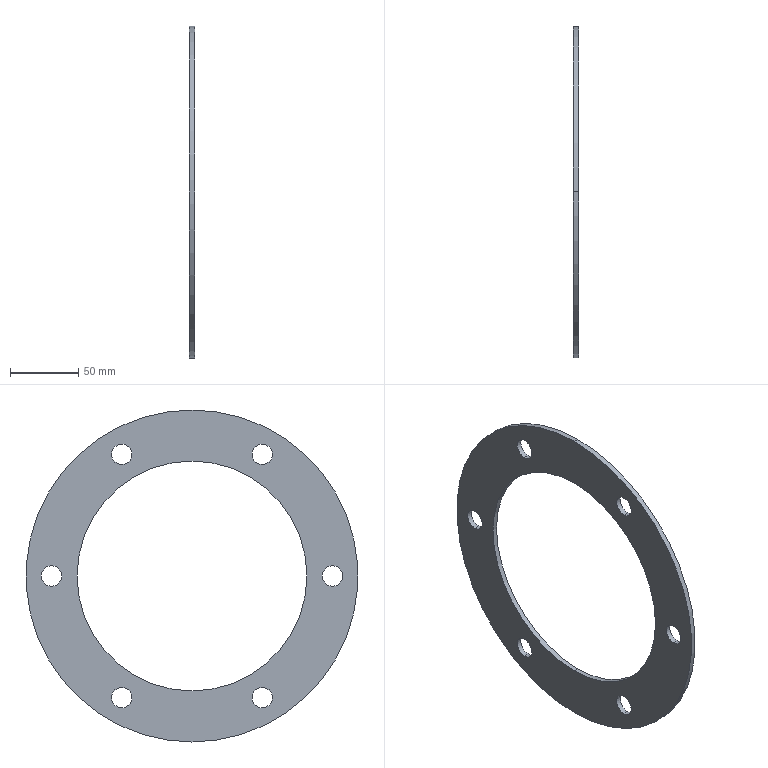Part | SolidWorks | features ICE 1, Revolution 1, Scale 1 | 1 solid | 18 faces | box 3.75 x 243.75 x 243.75 mm | volume 87142 mm3 | cylinder 16 | plane 2 | commonest cylinder face diameters 15 x12 168.75 x2 243.75 x2
STEP:
#1=CARTESIAN_POINT('',(-0.875,-103.125,7.5));
#2=VERTEX_POINT('',#1);
#3=CARTESIAN_POINT('',(-0.875,-103.125,-7.5));
#4=VERTEX_POINT('',#3);
#5=CARTESIAN_POINT('',(-0.875,-103.125,0.));
#6=DIRECTION('',(1.,0.,0.));
#7=DIRECTION('',(0.,0.,-1.));
#8=AXIS2_PLACEMENT_3D('',#5,#6,#7);
#9=CIRCLE('',#8,7.5);
#10=EDGE_CURVE('',#2,#4,#9,.T.);
#11=ORIENTED_EDGE('',*,*,#10,.F.);
#12=CARTESIAN_POINT('',(2.875,-103.125,7.5));
#13=VERTEX_POINT('',#12);
#14=CARTESIAN_POINT('',(-15.875,-103.125,7.5));
#15=DIRECTION('',(1.,0.,0.));
#16=VECTOR('',#15,1000.);
#17=LINE('',#14,#16);
#18=EDGE_CURVE('',#2,#13,#17,.T.);
#19=ORIENTED_EDGE('',*,*,#18,.T.);
#20=CARTESIAN_POINT('',(2.875,-103.125,-7.5));
#21=VERTEX_POINT('',#20);
#22=CARTESIAN_POINT('',(2.875,-103.125,0.));
#23=DIRECTION('',(1.,0.,0.));
#24=DIRECTION('',(0.,0.,1.));
#25=AXIS2_PLACEMENT_3D('',#22,#23,#24);
#26=CIRCLE('',#25,7.5);
#27=EDGE_CURVE('',#13,#21,#26,.T.);
#28=ORIENTED_EDGE('',*,*,#27,.T.);
#29=CARTESIAN_POINT('',(-15.875,-103.125,-7.5));
#30=DIRECTION('',(1.,0.,0.));
#31=VECTOR('',#30,1000.);
#32=LINE('',#29,#31);
#33=EDGE_CURVE('',#4,#21,#32,.T.);
#34=ORIENTED_EDGE('',*,*,#33,.F.);
#35=EDGE_LOOP('',(#11,#19,#28,#34));
#36=FACE_OUTER_BOUND('',#35,.T.);
#37=CARTESIAN_POINT('',(-15.875,-103.125,0.));
#38=DIRECTION('',(1.,0.,0.));
#39=DIRECTION('',(0.,0.,-1.));
#40=AXIS2_PLACEMENT_3D('',#37,#38,#39);
#41=CYLINDRICAL_SURFACE('',#40,7.5);
#42=ADVANCED_FACE('',(#36),#41,.F.);
#43=CARTESIAN_POINT('',(-0.875,-51.562,96.809));
#44=VERTEX_POINT('',#43);
#45=CARTESIAN_POINT('',(-0.875,-51.562,81.809));
#46=VERTEX_POINT('',#45);
#47=CARTESIAN_POINT('',(-0.875,-51.562,89.309));
#48=DIRECTION('',(1.,0.,0.));
#49=DIRECTION('',(0.,0.,-1.));
#50=AXIS2_PLACEMENT_3D('',#47,#48,#49);
#51=CIRCLE('',#50,7.5);
#52=EDGE_CURVE('',#44,#46,#51,.T.);
#53=ORIENTED_EDGE('',*,*,#52,.F.);
#54=CARTESIAN_POINT('',(2.875,-51.562,96.809));
#55=VERTEX_POINT('',#54);
#56=CARTESIAN_POINT('',(-15.875,-51.562,96.809));
#57=DIRECTION('',(1.,0.,0.));
#58=VECTOR('',#57,1000.);
#59=LINE('',#56,#58);
#60=EDGE_CURVE('',#44,#55,#59,.T.);
#61=ORIENTED_EDGE('',*,*,#60,.T.);
#62=CARTESIAN_POINT('',(2.875,-51.562,81.809));
#63=VERTEX_POINT('',#62);
#64=CARTESIAN_POINT('',(2.875,-51.562,89.309));
#65=DIRECTION('',(1.,0.,0.));
#66=DIRECTION('',(0.,0.,1.));
#67=AXIS2_PLACEMENT_3D('',#64,#65,#66);
#68=CIRCLE('',#67,7.5);
#69=EDGE_CURVE('',#55,#63,#68,.T.);
#70=ORIENTED_EDGE('',*,*,#69,.T.);
#71=CARTESIAN_POINT('',(-15.875,-51.562,81.809));
#72=DIRECTION('',(1.,0.,0.));
#73=VECTOR('',#72,1000.);
#74=LINE('',#71,#73);
#75=EDGE_CURVE('',#46,#63,#74,.T.);
#76=ORIENTED_EDGE('',*,*,#75,.F.);
#77=EDGE_LOOP('',(#53,#61,#70,#76));
#78=FACE_OUTER_BOUND('',#77,.T.);
#79=CARTESIAN_POINT('',(-15.875,-51.562,89.309));
#80=DIRECTION('',(1.,0.,0.));
#81=DIRECTION('',(0.,0.,-1.));
#82=AXIS2_PLACEMENT_3D('',#79,#80,#81);
#83=CYLINDRICAL_SURFACE('',#82,7.5);
#84=ADVANCED_FACE('',(#78),#83,.F.);
#85=CARTESIAN_POINT('',(-0.875,-51.562,-81.809));
#86=VERTEX_POINT('',#85);
#87=CARTESIAN_POINT('',(-0.875,-51.562,-96.809));
#88=VERTEX_POINT('',#87);
#89=CARTESIAN_POINT('',(-0.875,-51.562,-89.309));
#90=DIRECTION('',(1.,0.,0.));
#91=DIRECTION('',(0.,0.,-1.));
#92=AXIS2_PLACEMENT_3D('',#89,#90,#91);
#93=CIRCLE('',#92,7.5);
#94=EDGE_CURVE('',#86,#88,#93,.T.);
#95=ORIENTED_EDGE('',*,*,#94,.F.);
#96=CARTESIAN_POINT('',(2.875,-51.562,-81.809));
#97=VERTEX_POINT('',#96);
#98=CARTESIAN_POINT('',(-15.875,-51.562,-81.809));
#99=DIRECTION('',(1.,0.,0.));
#100=VECTOR('',#99,1000.);
#101=LINE('',#98,#100);
#102=EDGE_CURVE('',#86,#97,#101,.T.);
#103=ORIENTED_EDGE('',*,*,#102,.T.);
#104=CARTESIAN_POINT('',(2.875,-51.562,-96.809));
#105=VERTEX_POINT('',#104);
#106=CARTESIAN_POINT('',(2.875,-51.562,-89.309));
#107=DIRECTION('',(1.,0.,0.));
#108=DIRECTION('',(0.,0.,1.));
#109=AXIS2_PLACEMENT_3D('',#106,#107,#108);
#110=CIRCLE('',#109,7.5);
#111=EDGE_CURVE('',#97,#105,#110,.T.);
#112=ORIENTED_EDGE('',*,*,#111,.T.);
#113=CARTESIAN_POINT('',(-15.875,-51.562,-96.809));
#114=DIRECTION('',(1.,0.,0.));
#115=VECTOR('',#114,1000.);
#116=LINE('',#113,#115);
#117=EDGE_CURVE('',#88,#105,#116,.T.);
#118=ORIENTED_EDGE('',*,*,#117,.F.);
#119=EDGE_LOOP('',(#95,#103,#112,#118));
#120=FACE_OUTER_BOUND('',#119,.T.);
#121=CARTESIAN_POINT('',(-15.875,-51.562,-89.309));
#122=DIRECTION('',(1.,0.,0.));
#123=DIRECTION('',(0.,0.,-1.));
#124=AXIS2_PLACEMENT_3D('',#121,#122,#123);
#125=CYLINDRICAL_SURFACE('',#124,7.5);
#126=ADVANCED_FACE('',(#120),#125,.F.);
#127=CARTESIAN_POINT('',(-0.875,51.562,96.809));
#128=VERTEX_POINT('',#127);
#129=CARTESIAN_POINT('',(-0.875,51.562,81.809));
#130=VERTEX_POINT('',#129);
#131=CARTESIAN_POINT('',(-0.875,51.562,89.309));
#132=DIRECTION('',(1.,0.,0.));
#133=DIRECTION('',(0.,0.,-1.));
#134=AXIS2_PLACEMENT_3D('',#131,#132,#133);
#135=CIRCLE('',#134,7.5);
#136=EDGE_CURVE('',#128,#130,#135,.T.);
#137=ORIENTED_EDGE('',*,*,#136,.F.);
#138=CARTESIAN_POINT('',(2.875,51.562,96.809));
#139=VERTEX_POINT('',#138);
#140=CARTESIAN_POINT('',(-15.875,51.562,96.809));
#141=DIRECTION('',(1.,0.,0.));
#142=VECTOR('',#141,1000.);
#143=LINE('',#140,#142);
#144=EDGE_CURVE('',#128,#139,#143,.T.);
#145=ORIENTED_EDGE('',*,*,#144,.T.);
#146=CARTESIAN_POINT('',(2.875,51.562,81.809));
#147=VERTEX_POINT('',#146);
#148=CARTESIAN_POINT('',(2.875,51.562,89.309));
#149=DIRECTION('',(1.,0.,0.));
#150=DIRECTION('',(0.,0.,-1.));
#151=AXIS2_PLACEMENT_3D('',#148,#149,#150);
#152=CIRCLE('',#151,7.5);
#153=EDGE_CURVE('',#139,#147,#152,.T.);
#154=ORIENTED_EDGE('',*,*,#153,.T.);
#155=CARTESIAN_POINT('',(-15.875,51.562,81.809));
#156=DIRECTION('',(1.,0.,0.));
#157=VECTOR('',#156,1000.);
#158=LINE('',#155,#157);
#159=EDGE_CURVE('',#130,#147,#158,.T.);
#160=ORIENTED_EDGE('',*,*,#159,.F.);
#161=EDGE_LOOP('',(#137,#145,#154,#160));
#162=FACE_OUTER_BOUND('',#161,.T.);
#163=CARTESIAN_POINT('',(-15.875,51.562,89.309));
#164=DIRECTION('',(1.,0.,0.));
#165=DIRECTION('',(0.,0.,-1.));
#166=AXIS2_PLACEMENT_3D('',#163,#164,#165);
#167=CYLINDRICAL_SURFACE('',#166,7.5);
#168=ADVANCED_FACE('',(#162),#167,.F.);
#169=CARTESIAN_POINT('',(-0.875,51.562,-81.809));
#170=VERTEX_POINT('',#169);
#171=CARTESIAN_POINT('',(-0.875,51.562,-96.809));
#172=VERTEX_POINT('',#171);
#173=CARTESIAN_POINT('',(-0.875,51.562,-89.309));
#174=DIRECTION('',(1.,0.,0.));
#175=DIRECTION('',(0.,0.,-1.));
#176=AXIS2_PLACEMENT_3D('',#173,#174,#175);
#177=CIRCLE('',#176,7.5);
#178=EDGE_CURVE('',#170,#172,#177,.T.);
#179=ORIENTED_EDGE('',*,*,#178,.F.);
#180=CARTESIAN_POINT('',(2.875,51.562,-81.809));
#181=VERTEX_POINT('',#180);
#182=CARTESIAN_POINT('',(-15.875,51.562,-81.809));
#183=DIRECTION('',(1.,0.,0.));
#184=VECTOR('',#183,1000.);
#185=LINE('',#182,#184);
#186=EDGE_CURVE('',#170,#181,#185,.T.);
#187=ORIENTED_EDGE('',*,*,#186,.T.);
#188=CARTESIAN_POINT('',(2.875,51.562,-96.809));
#189=VERTEX_POINT('',#188);
#190=CARTESIAN_POINT('',(2.875,51.562,-89.309));
#191=DIRECTION('',(1.,0.,0.));
#192=DIRECTION('',(0.,0.,-1.));
#193=AXIS2_PLACEMENT_3D('',#190,#191,#192);
#194=CIRCLE('',#193,7.5);
#195=EDGE_CURVE('',#181,#189,#194,.T.);
#196=ORIENTED_EDGE('',*,*,#195,.T.);
#197=CARTESIAN_POINT('',(-15.875,51.562,-96.809));
#198=DIRECTION('',(1.,0.,0.));
#199=VECTOR('',#198,1000.);
#200=LINE('',#197,#199);
#201=EDGE_CURVE('',#172,#189,#200,.T.);
#202=ORIENTED_EDGE('',*,*,#201,.F.);
#203=EDGE_LOOP('',(#179,#187,#196,#202));
#204=FACE_OUTER_BOUND('',#203,.T.);
#205=CARTESIAN_POINT('',(-15.875,51.562,-89.309));
#206=DIRECTION('',(1.,0.,0.));
#207=DIRECTION('',(0.,0.,-1.));
#208=AXIS2_PLACEMENT_3D('',#205,#206,#207);
#209=CYLINDRICAL_SURFACE('',#208,7.5);
#210=ADVANCED_FACE('',(#204),#209,.F.);
#211=CARTESIAN_POINT('',(-0.875,103.125,7.5));
#212=VERTEX_POINT('',#211);
#213=CARTESIAN_POINT('',(-0.875,103.125,-7.5));
#214=VERTEX_POINT('',#213);
#215=CARTESIAN_POINT('',(-0.875,103.125,0.));
#216=DIRECTION('',(1.,0.,0.));
#217=DIRECTION('',(0.,0.,-1.));
#218=AXIS2_PLACEMENT_3D('',#215,#216,#217);
#219=CIRCLE('',#218,7.5);
#220=EDGE_CURVE('',#212,#214,#219,.T.);
#221=ORIENTED_EDGE('',*,*,#220,.F.);
#222=CARTESIAN_POINT('',(2.875,103.125,7.5));
#223=VERTEX_POINT('',#222);
#224=CARTESIAN_POINT('',(-15.875,103.125,7.5));
#225=DIRECTION('',(1.,0.,0.));
#226=VECTOR('',#225,1000.);
#227=LINE('',#224,#226);
#228=EDGE_CURVE('',#212,#223,#227,.T.);
#229=ORIENTED_EDGE('',*,*,#228,.T.);
#230=CARTESIAN_POINT('',(2.875,103.125,-7.5));
#231=VERTEX_POINT('',#230);
#232=CARTESIAN_POINT('',(2.875,103.125,0.));
#233=DIRECTION('',(1.,0.,0.));
#234=DIRECTION('',(0.,0.,-1.));
#235=AXIS2_PLACEMENT_3D('',#232,#233,#234);
#236=CIRCLE('',#235,7.5);
#237=EDGE_CURVE('',#223,#231,#236,.T.);
#238=ORIENTED_EDGE('',*,*,#237,.T.);
#239=CARTESIAN_POINT('',(-15.875,103.125,-7.5));
#240=DIRECTION('',(1.,0.,0.));
#241=VECTOR('',#240,1000.);
#242=LINE('',#239,#241);
#243=EDGE_CURVE('',#214,#231,#242,.T.);
#244=ORIENTED_EDGE('',*,*,#243,.F.);
#245=EDGE_LOOP('',(#221,#229,#238,#244));
#246=FACE_OUTER_BOUND('',#245,.T.);
#247=CARTESIAN_POINT('',(-15.875,103.125,0.));
#248=DIRECTION('',(1.,0.,0.));
#249=DIRECTION('',(0.,0.,-1.));
#250=AXIS2_PLACEMENT_3D('',#247,#248,#249);
#251=CYLINDRICAL_SURFACE('',#250,7.5);
#252=ADVANCED_FACE('',(#246),#251,.F.);
#253=CARTESIAN_POINT('',(2.875,0.,121.875));
#254=VERTEX_POINT('',#253);
#255=CARTESIAN_POINT('',(2.875,0.,-121.875));
#256=VERTEX_POINT('',#255);
#257=CARTESIAN_POINT('',(2.875,0.,0.));
#258=DIRECTION('',(-1.,0.,0.));
#259=DIRECTION('',(0.,0.,1.));
#260=AXIS2_PLACEMENT_3D('',#257,#258,#259);
#261=CIRCLE('',#260,121.875);
#262=EDGE_CURVE('',#254,#256,#261,.T.);
#263=ORIENTED_EDGE('',*,*,#262,.T.);
#264=CARTESIAN_POINT('',(-0.875,0.,-121.875));
#265=VERTEX_POINT('',#264);
#266=CARTESIAN_POINT('',(-0.875,0.,-121.875));
#267=DIRECTION('',(-1.,0.,0.));
#268=VECTOR('',#267,1000.);
#269=LINE('',#266,#268);
#270=EDGE_CURVE('',#256,#265,#269,.T.);
#271=ORIENTED_EDGE('',*,*,#270,.T.);
#272=CARTESIAN_POINT('',(-0.875,0.,121.875));
#273=VERTEX_POINT('',#272);
#274=CARTESIAN_POINT('',(-0.875,0.,0.));
#275=DIRECTION('',(-1.,0.,0.));
#276=DIRECTION('',(0.,0.,1.));
#277=AXIS2_PLACEMENT_3D('',#274,#275,#276);
#278=CIRCLE('',#277,121.875);
#279=EDGE_CURVE('',#273,#265,#278,.T.);
#280=ORIENTED_EDGE('',*,*,#279,.F.);
#281=CARTESIAN_POINT('',(-0.875,0.,121.875));
#282=DIRECTION('',(-1.,0.,0.));
#283=VECTOR('',#282,1000.);
#284=LINE('',#281,#283);
#285=EDGE_CURVE('',#254,#273,#284,.T.);
#286=ORIENTED_EDGE('',*,*,#285,.F.);
#287=EDGE_LOOP('',(#263,#271,#280,#286));
#288=FACE_OUTER_BOUND('',#287,.T.);
#289=CARTESIAN_POINT('',(-0.875,0.,0.));
#290=DIRECTION('',(-1.,0.,0.));
#291=DIRECTION('',(0.,0.,1.));
#292=AXIS2_PLACEMENT_3D('',#289,#290,#291);
#293=CYLINDRICAL_SURFACE('',#292,121.875);
#294=ADVANCED_FACE('',(#288),#293,.T.);
#295=CARTESIAN_POINT('',(2.875,0.,-84.375));
#296=VERTEX_POINT('',#295);
#297=CARTESIAN_POINT('',(2.875,0.,84.375));
#298=VERTEX_POINT('',#297);
#299=CARTESIAN_POINT('',(2.875,0.,0.));
#300=DIRECTION('',(-1.,0.,0.));
#301=DIRECTION('',(0.,0.,1.));
#302=AXIS2_PLACEMENT_3D('',#299,#300,#301);
#303=CIRCLE('',#302,84.375);
#304=EDGE_CURVE('',#296,#298,#303,.T.);
#305=ORIENTED_EDGE('',*,*,#304,.F.);
#306=CARTESIAN_POINT('',(-0.875,0.,-84.375));
#307=VERTEX_POINT('',#306);
#308=CARTESIAN_POINT('',(-0.875,0.,-84.375));
#309=DIRECTION('',(-1.,0.,0.));
#310=VECTOR('',#309,1000.);
#311=LINE('',#308,#310);
#312=EDGE_CURVE('',#296,#307,#311,.T.);
#313=ORIENTED_EDGE('',*,*,#312,.T.);
#314=CARTESIAN_POINT('',(-0.875,0.,84.375));
#315=VERTEX_POINT('',#314);
#316=CARTESIAN_POINT('',(-0.875,0.,0.));
#317=DIRECTION('',(-1.,0.,0.));
#318=DIRECTION('',(0.,0.,1.));
#319=AXIS2_PLACEMENT_3D('',#316,#317,#318);
#320=CIRCLE('',#319,84.375);
#321=EDGE_CURVE('',#307,#315,#320,.T.);
#322=ORIENTED_EDGE('',*,*,#321,.T.);
#323=CARTESIAN_POINT('',(-0.875,0.,84.375));
#324=DIRECTION('',(-1.,0.,0.));
#325=VECTOR('',#324,1000.);
#326=LINE('',#323,#325);
#327=EDGE_CURVE('',#298,#315,#326,.T.);
#328=ORIENTED_EDGE('',*,*,#327,.F.);
#329=EDGE_LOOP('',(#305,#313,#322,#328));
#330=FACE_OUTER_BOUND('',#329,.T.);
#331=CARTESIAN_POINT('',(-0.875,0.,0.));
#332=DIRECTION('',(-1.,0.,0.));
#333=DIRECTION('',(0.,0.,1.));
#334=AXIS2_PLACEMENT_3D('',#331,#332,#333);
#335=CYLINDRICAL_SURFACE('',#334,84.375);
#336=ADVANCED_FACE('',(#330),#335,.F.);
#337=CARTESIAN_POINT('',(-0.875,-103.125,0.));
#338=DIRECTION('',(1.,0.,0.));
#339=DIRECTION('',(0.,0.,-1.));
#340=AXIS2_PLACEMENT_3D('',#337,#338,#339);
#341=CIRCLE('',#340,7.5);
#342=EDGE_CURVE('',#4,#2,#341,.T.);
#343=ORIENTED_EDGE('',*,*,#342,.T.);
#344=ORIENTED_EDGE('',*,*,#10,.T.);
#345=EDGE_LOOP('',(#343,#344));
#346=FACE_BOUND('',#345,.T.);
#347=CARTESIAN_POINT('',(-0.875,-51.562,89.309));
#348=DIRECTION('',(1.,0.,0.));
#349=DIRECTION('',(0.,0.,-1.));
#350=AXIS2_PLACEMENT_3D('',#347,#348,#349);
#351=CIRCLE('',#350,7.5);
#352=EDGE_CURVE('',#46,#44,#351,.T.);
#353=ORIENTED_EDGE('',*,*,#352,.T.);
#354=ORIENTED_EDGE('',*,*,#52,.T.);
#355=EDGE_LOOP('',(#353,#354));
#356=FACE_BOUND('',#355,.T.);
#357=CARTESIAN_POINT('',(-0.875,-51.562,-89.309));
#358=DIRECTION('',(1.,0.,0.));
#359=DIRECTION('',(0.,0.,-1.));
#360=AXIS2_PLACEMENT_3D('',#357,#358,#359);
#361=CIRCLE('',#360,7.5);
#362=EDGE_CURVE('',#88,#86,#361,.T.);
#363=ORIENTED_EDGE('',*,*,#362,.T.);
#364=ORIENTED_EDGE('',*,*,#94,.T.);
#365=EDGE_LOOP('',(#363,#364));
#366=FACE_BOUND('',#365,.T.);
#367=CARTESIAN_POINT('',(-0.875,51.562,89.309));
#368=DIRECTION('',(1.,0.,0.));
#369=DIRECTION('',(0.,0.,-1.));
#370=AXIS2_PLACEMENT_3D('',#367,#368,#369);
#371=CIRCLE('',#370,7.5);
#372=EDGE_CURVE('',#130,#128,#371,.T.);
#373=ORIENTED_EDGE('',*,*,#372,.T.);
#374=ORIENTED_EDGE('',*,*,#136,.T.);
#375=EDGE_LOOP('',(#373,#374));
#376=FACE_BOUND('',#375,.T.);
#377=CARTESIAN_POINT('',(-0.875,51.562,-89.309));
#378=DIRECTION('',(1.,0.,0.));
#379=DIRECTION('',(0.,0.,-1.));
#380=AXIS2_PLACEMENT_3D('',#377,#378,#379);
#381=CIRCLE('',#380,7.5);
#382=EDGE_CURVE('',#172,#170,#381,.T.);
#383=ORIENTED_EDGE('',*,*,#382,.T.);
#384=ORIENTED_EDGE('',*,*,#178,.T.);
#385=EDGE_LOOP('',(#383,#384));
#386=FACE_BOUND('',#385,.T.);
#387=CARTESIAN_POINT('',(-0.875,103.125,0.));
#388=DIRECTION('',(1.,0.,0.));
#389=DIRECTION('',(0.,0.,-1.));
#390=AXIS2_PLACEMENT_3D('',#387,#388,#389);
#391=CIRCLE('',#390,7.5);
#392=EDGE_CURVE('',#214,#212,#391,.T.);
#393=ORIENTED_EDGE('',*,*,#392,.T.);
#394=ORIENTED_EDGE('',*,*,#220,.T.);
#395=EDGE_LOOP('',(#393,#394));
#396=FACE_BOUND('',#395,.T.);
#397=CARTESIAN_POINT('',(-0.875,0.,0.));
#398=DIRECTION('',(-1.,0.,0.));
#399=DIRECTION('',(0.,0.,1.));
#400=AXIS2_PLACEMENT_3D('',#397,#398,#399);
#401=CIRCLE('',#400,84.375);
#402=EDGE_CURVE('',#315,#307,#401,.T.);
#403=ORIENTED_EDGE('',*,*,#402,.F.);
#404=ORIENTED_EDGE('',*,*,#321,.F.);
#405=EDGE_LOOP('',(#403,#404));
#406=FACE_BOUND('',#405,.T.);
#407=ORIENTED_EDGE('',*,*,#279,.T.);
#408=CARTESIAN_POINT('',(-0.875,0.,0.));
#409=DIRECTION('',(-1.,0.,0.));
#410=DIRECTION('',(0.,0.,1.));
#411=AXIS2_PLACEMENT_3D('',#408,#409,#410);
#412=CIRCLE('',#411,121.875);
#413=EDGE_CURVE('',#265,#273,#412,.T.);
#414=ORIENTED_EDGE('',*,*,#413,.T.);
#415=EDGE_LOOP('',(#407,#414));
#416=FACE_OUTER_BOUND('',#415,.T.);
#417=CARTESIAN_POINT('',(-0.875,121.875,0.));
#418=DIRECTION('',(1.,0.,0.));
#419=DIRECTION('',(0.,0.,-1.));
#420=AXIS2_PLACEMENT_3D('',#417,#418,#419);
#421=PLANE('',#420);
#422=ADVANCED_FACE('',(#346,#356,#366,#376,#386,#396,#406,#416),#421,.F.);
#423=ORIENTED_EDGE('',*,*,#312,.F.);
#424=CARTESIAN_POINT('',(2.875,0.,0.));
#425=DIRECTION('',(-1.,0.,0.));
#426=DIRECTION('',(0.,0.,1.));
#427=AXIS2_PLACEMENT_3D('',#424,#425,#426);
#428=CIRCLE('',#427,84.375);
#429=EDGE_CURVE('',#298,#296,#428,.T.);
#430=ORIENTED_EDGE('',*,*,#429,.F.);
#431=ORIENTED_EDGE('',*,*,#327,.T.);
#432=ORIENTED_EDGE('',*,*,#402,.T.);
#433=EDGE_LOOP('',(#423,#430,#431,#432));
#434=FACE_OUTER_BOUND('',#433,.T.);
#435=CARTESIAN_POINT('',(-0.875,0.,0.));
#436=DIRECTION('',(-1.,0.,0.));
#437=DIRECTION('',(0.,0.,1.));
#438=AXIS2_PLACEMENT_3D('',#435,#436,#437);
#439=CYLINDRICAL_SURFACE('',#438,84.375);
#440=ADVANCED_FACE('',(#434),#439,.F.);
#441=CARTESIAN_POINT('',(2.875,-103.125,0.));
#442=DIRECTION('',(1.,0.,0.));
#443=DIRECTION('',(0.,0.,1.));
#444=AXIS2_PLACEMENT_3D('',#441,#442,#443);
#445=CIRCLE('',#444,7.5);
#446=EDGE_CURVE('',#21,#13,#445,.T.);
#447=ORIENTED_EDGE('',*,*,#446,.F.);
#448=ORIENTED_EDGE('',*,*,#27,.F.);
#449=EDGE_LOOP('',(#447,#448));
#450=FACE_BOUND('',#449,.T.);
#451=CARTESIAN_POINT('',(2.875,-51.562,89.309));
#452=DIRECTION('',(1.,0.,0.));
#453=DIRECTION('',(0.,0.,1.));
#454=AXIS2_PLACEMENT_3D('',#451,#452,#453);
#455=CIRCLE('',#454,7.5);
#456=EDGE_CURVE('',#63,#55,#455,.T.);
#457=ORIENTED_EDGE('',*,*,#456,.F.);
#458=ORIENTED_EDGE('',*,*,#69,.F.);
#459=EDGE_LOOP('',(#457,#458));
#460=FACE_BOUND('',#459,.T.);
#461=CARTESIAN_POINT('',(2.875,-51.562,-89.309));
#462=DIRECTION('',(1.,0.,0.));
#463=DIRECTION('',(0.,0.,1.));
#464=AXIS2_PLACEMENT_3D('',#461,#462,#463);
#465=CIRCLE('',#464,7.5);
#466=EDGE_CURVE('',#105,#97,#465,.T.);
#467=ORIENTED_EDGE('',*,*,#466,.F.);
#468=ORIENTED_EDGE('',*,*,#111,.F.);
#469=EDGE_LOOP('',(#467,#468));
#470=FACE_BOUND('',#469,.T.);
#471=CARTESIAN_POINT('',(2.875,51.562,89.309));
#472=DIRECTION('',(1.,0.,0.));
#473=DIRECTION('',(0.,0.,-1.));
#474=AXIS2_PLACEMENT_3D('',#471,#472,#473);
#475=CIRCLE('',#474,7.5);
#476=EDGE_CURVE('',#147,#139,#475,.T.);
#477=ORIENTED_EDGE('',*,*,#476,.F.);
#478=ORIENTED_EDGE('',*,*,#153,.F.);
#479=EDGE_LOOP('',(#477,#478));
#480=FACE_BOUND('',#479,.T.);
#481=CARTESIAN_POINT('',(2.875,51.562,-89.309));
#482=DIRECTION('',(1.,0.,0.));
#483=DIRECTION('',(0.,0.,-1.));
#484=AXIS2_PLACEMENT_3D('',#481,#482,#483);
#485=CIRCLE('',#484,7.5);
#486=EDGE_CURVE('',#189,#181,#485,.T.);
#487=ORIENTED_EDGE('',*,*,#486,.F.);
#488=ORIENTED_EDGE('',*,*,#195,.F.);
#489=EDGE_LOOP('',(#487,#488));
#490=FACE_BOUND('',#489,.T.);
#491=CARTESIAN_POINT('',(2.875,103.125,0.));
#492=DIRECTION('',(1.,0.,0.));
#493=DIRECTION('',(0.,0.,-1.));
#494=AXIS2_PLACEMENT_3D('',#491,#492,#493);
#495=CIRCLE('',#494,7.5);
#496=EDGE_CURVE('',#231,#223,#495,.T.);
#497=ORIENTED_EDGE('',*,*,#496,.F.);
#498=ORIENTED_EDGE('',*,*,#237,.F.);
#499=EDGE_LOOP('',(#497,#498));
#500=FACE_BOUND('',#499,.T.);
#501=ORIENTED_EDGE('',*,*,#262,.F.);
#502=CARTESIAN_POINT('',(2.875,0.,0.));
#503=DIRECTION('',(-1.,0.,0.));
#504=DIRECTION('',(0.,0.,1.));
#505=AXIS2_PLACEMENT_3D('',#502,#503,#504);
#506=CIRCLE('',#505,121.875);
#507=EDGE_CURVE('',#256,#254,#506,.T.);
#508=ORIENTED_EDGE('',*,*,#507,.F.);
#509=EDGE_LOOP('',(#501,#508));
#510=FACE_OUTER_BOUND('',#509,.T.);
#511=ORIENTED_EDGE('',*,*,#429,.T.);
#512=ORIENTED_EDGE('',*,*,#304,.T.);
#513=EDGE_LOOP('',(#511,#512));
#514=FACE_BOUND('',#513,.T.);
#515=CARTESIAN_POINT('',(2.875,121.875,0.));
#516=DIRECTION('',(-1.,0.,0.));
#517=DIRECTION('',(0.,0.,1.));
#518=AXIS2_PLACEMENT_3D('',#515,#516,#517);
#519=PLANE('',#518);
#520=ADVANCED_FACE('',(#450,#460,#470,#480,#490,#500,#510,#514),#519,.F.);
#521=ORIENTED_EDGE('',*,*,#270,.F.);
#522=ORIENTED_EDGE('',*,*,#507,.T.);
#523=ORIENTED_EDGE('',*,*,#285,.T.);
#524=ORIENTED_EDGE('',*,*,#413,.F.);
#525=EDGE_LOOP('',(#521,#522,#523,#524));
#526=FACE_OUTER_BOUND('',#525,.T.);
#527=CARTESIAN_POINT('',(-0.875,0.,0.));
#528=DIRECTION('',(-1.,0.,0.));
#529=DIRECTION('',(0.,0.,1.));
#530=AXIS2_PLACEMENT_3D('',#527,#528,#529);
#531=CYLINDRICAL_SURFACE('',#530,121.875);
#532=ADVANCED_FACE('',(#526),#531,.T.);
#533=ORIENTED_EDGE('',*,*,#228,.F.);
#534=ORIENTED_EDGE('',*,*,#392,.F.);
#535=ORIENTED_EDGE('',*,*,#243,.T.);
#536=ORIENTED_EDGE('',*,*,#496,.T.);
#537=EDGE_LOOP('',(#533,#534,#535,#536));
#538=FACE_OUTER_BOUND('',#537,.T.);
#539=CARTESIAN_POINT('',(-15.875,103.125,0.));
#540=DIRECTION('',(1.,0.,0.));
#541=DIRECTION('',(0.,0.,-1.));
#542=AXIS2_PLACEMENT_3D('',#539,#540,#541);
#543=CYLINDRICAL_SURFACE('',#542,7.5);
#544=ADVANCED_FACE('',(#538),#543,.F.);
#545=ORIENTED_EDGE('',*,*,#186,.F.);
#546=ORIENTED_EDGE('',*,*,#382,.F.);
#547=ORIENTED_EDGE('',*,*,#201,.T.);
#548=ORIENTED_EDGE('',*,*,#486,.T.);
#549=EDGE_LOOP('',(#545,#546,#547,#548));
#550=FACE_OUTER_BOUND('',#549,.T.);
#551=CARTESIAN_POINT('',(-15.875,51.562,-89.309));
#552=DIRECTION('',(1.,0.,0.));
#553=DIRECTION('',(0.,0.,-1.));
#554=AXIS2_PLACEMENT_3D('',#551,#552,#553);
#555=CYLINDRICAL_SURFACE('',#554,7.5);
#556=ADVANCED_FACE('',(#550),#555,.F.);
#557=ORIENTED_EDGE('',*,*,#144,.F.);
#558=ORIENTED_EDGE('',*,*,#372,.F.);
#559=ORIENTED_EDGE('',*,*,#159,.T.);
#560=ORIENTED_EDGE('',*,*,#476,.T.);
#561=EDGE_LOOP('',(#557,#558,#559,#560));
#562=FACE_OUTER_BOUND('',#561,.T.);
#563=CARTESIAN_POINT('',(-15.875,51.562,89.309));
#564=DIRECTION('',(1.,0.,0.));
#565=DIRECTION('',(0.,0.,-1.));
#566=AXIS2_PLACEMENT_3D('',#563,#564,#565);
#567=CYLINDRICAL_SURFACE('',#566,7.5);
#568=ADVANCED_FACE('',(#562),#567,.F.);
#569=ORIENTED_EDGE('',*,*,#102,.F.);
#570=ORIENTED_EDGE('',*,*,#362,.F.);
#571=ORIENTED_EDGE('',*,*,#117,.T.);
#572=ORIENTED_EDGE('',*,*,#466,.T.);
#573=EDGE_LOOP('',(#569,#570,#571,#572));
#574=FACE_OUTER_BOUND('',#573,.T.);
#575=CARTESIAN_POINT('',(-15.875,-51.562,-89.309));
#576=DIRECTION('',(1.,0.,0.));
#577=DIRECTION('',(0.,0.,-1.));
#578=AXIS2_PLACEMENT_3D('',#575,#576,#577);
#579=CYLINDRICAL_SURFACE('',#578,7.5);
#580=ADVANCED_FACE('',(#574),#579,.F.);
#581=ORIENTED_EDGE('',*,*,#60,.F.);
#582=ORIENTED_EDGE('',*,*,#352,.F.);
#583=ORIENTED_EDGE('',*,*,#75,.T.);
#584=ORIENTED_EDGE('',*,*,#456,.T.);
#585=EDGE_LOOP('',(#581,#582,#583,#584));
#586=FACE_OUTER_BOUND('',#585,.T.);
#587=CARTESIAN_POINT('',(-15.875,-51.562,89.309));
#588=DIRECTION('',(1.,0.,0.));
#589=DIRECTION('',(0.,0.,-1.));
#590=AXIS2_PLACEMENT_3D('',#587,#588,#589);
#591=CYLINDRICAL_SURFACE('',#590,7.5);
#592=ADVANCED_FACE('',(#586),#591,.F.);
#593=ORIENTED_EDGE('',*,*,#18,.F.);
#594=ORIENTED_EDGE('',*,*,#342,.F.);
#595=ORIENTED_EDGE('',*,*,#33,.T.);
#596=ORIENTED_EDGE('',*,*,#446,.T.);
#597=EDGE_LOOP('',(#593,#594,#595,#596));
#598=FACE_OUTER_BOUND('',#597,.T.);
#599=CARTESIAN_POINT('',(-15.875,-103.125,0.));
#600=DIRECTION('',(1.,0.,0.));
#601=DIRECTION('',(0.,0.,-1.));
#602=AXIS2_PLACEMENT_3D('',#599,#600,#601);
#603=CYLINDRICAL_SURFACE('',#602,7.5);
#604=ADVANCED_FACE('',(#598),#603,.F.);
#605=CLOSED_SHELL('',(#42,#84,#126,#168,#210,#252,#294,#336,#422,#440,#520,#532,#544,#556,#568,#580,#592,#604));
#606=MANIFOLD_SOLID_BREP('',#605);
#607=CARTESIAN_POINT('',(0.,0.,0.));
#608=DIRECTION('',(0.,0.,1.));
#609=DIRECTION('',(1.,0.,0.));
#610=AXIS2_PLACEMENT_3D('',#607,#608,#609);
#611=(LENGTH_UNIT()NAMED_UNIT(*)SI_UNIT(.MILLI.,.METRE.));
#612=UNCERTAINTY_MEASURE_WITH_UNIT(LENGTH_MEASURE(0.00001),#611,'','');
#613=(NAMED_UNIT(*)PLANE_ANGLE_UNIT()SI_UNIT($,.RADIAN.));
#614=(NAMED_UNIT(*)SI_UNIT($,.STERADIAN.)SOLID_ANGLE_UNIT());
#615=(GEOMETRIC_REPRESENTATION_CONTEXT(3)GLOBAL_UNCERTAINTY_ASSIGNED_CONTEXT((#612))GLOBAL_UNIT_ASSIGNED_CONTEXT((#611,#613,#614))REPRESENTATION_CONTEXT('',''));
#616=ADVANCED_BREP_SHAPE_REPRESENTATION('',(#606,#610),#615);